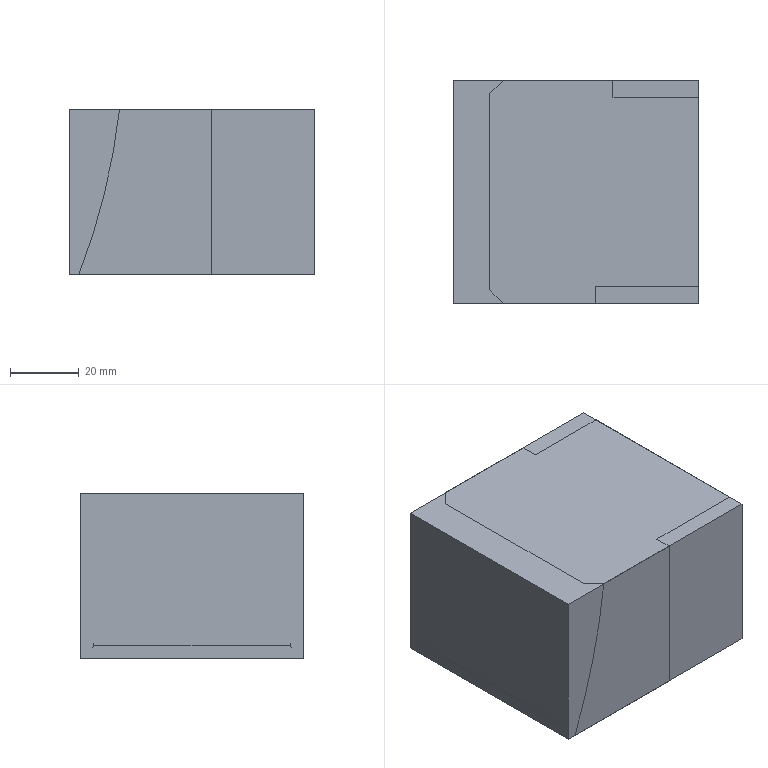NC program | NX | posted with a generic post | part box 71.51 x 65 x 48 mm
Lines 1 to 20 of 3379:
N10 G17 G21 G94 G90
(FLOOR_WALL , TOOL : D63)
N12 T01 M6
N14 G54
N16 G17 G0 G90 X-73.255 Y35.497 B0. C0. S6500 M3
N18 G43 Z30. H1
N20 Z3.
N22 G94 G1 Z0. F1250.
N24 X-70.255
N26 X70.255
N28 Y-10.3
N30 X-70.255
N32 X-73.255
N34 Z3.
N36 G0 Z30.
N38 M5